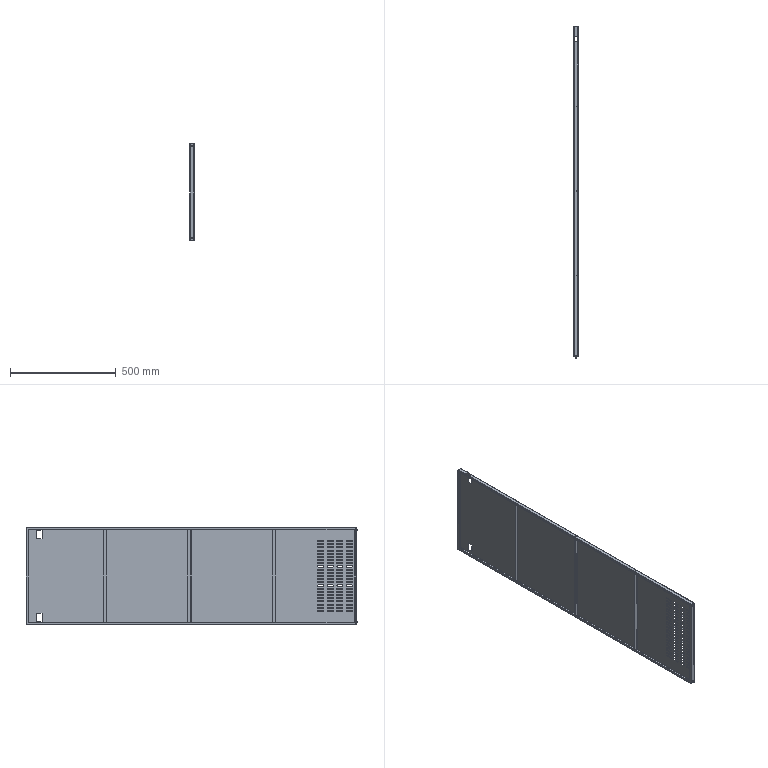Part | SolidWorks | features CompositeCurve 2 | 7 solids | 994 faces | box 20 x 1568 x 458 mm | volume 1656594 mm3 | plane 516 | cylinder 430 | spline 32 | torus 16 | commonest cylinder face diameters 5 x368 0.2 x23 2.2 x19 4 x8 4.5 x8 8 x4